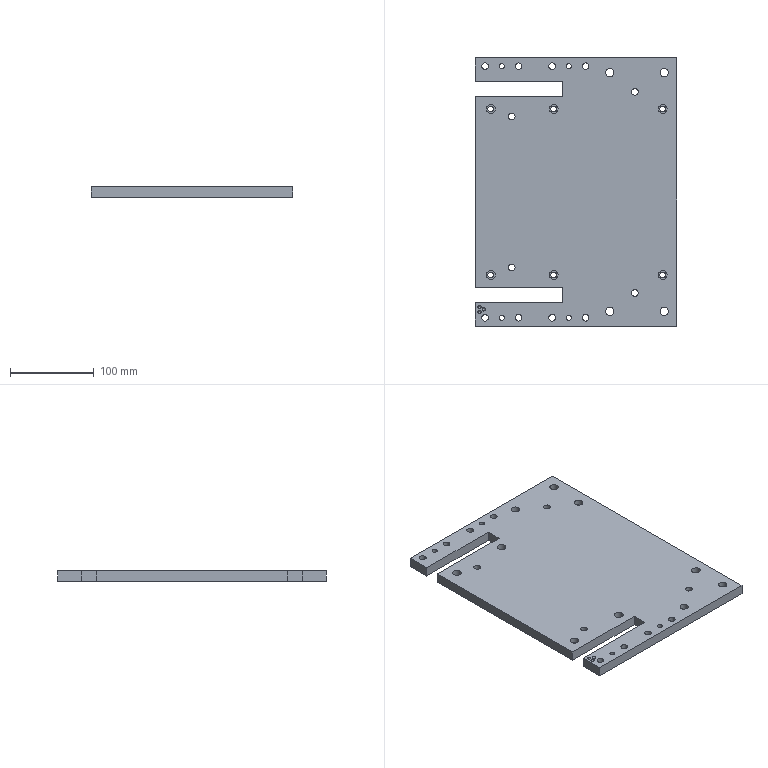Part | STEP file | 200 mesh_id2086 | 1 solid | 55 faces | box 240 x 320 x 12 mm | volume 859349 mm3 | cylinder 32 | plane 20 | cone 3 | commonest cylinder face diameters 8 x8 7 x6 10.5 x6 6.01 x4 8.01 x4 10 x4